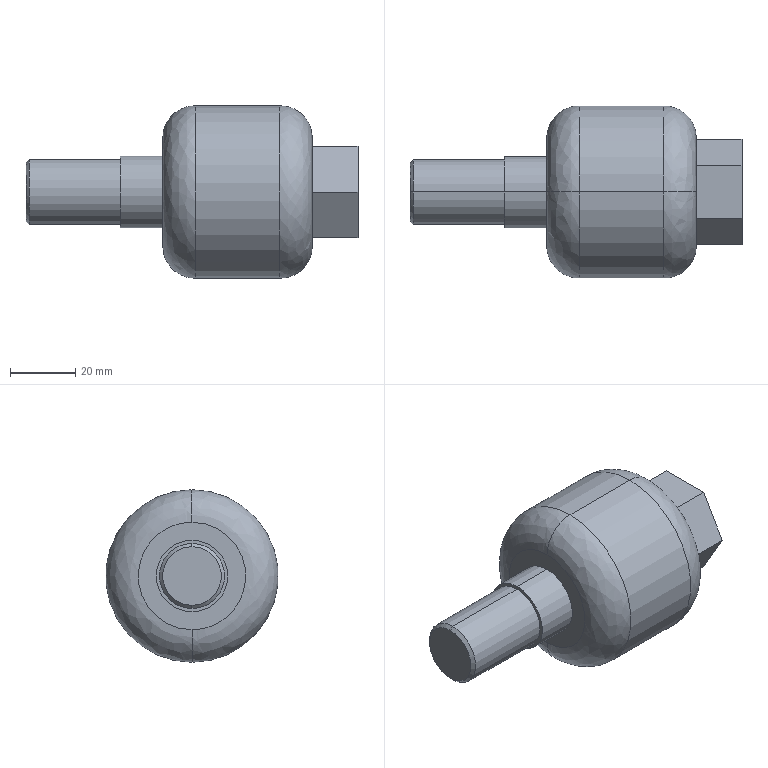Part | STEP file | FJ1020 Floating Joint | 1 solid | 26 faces | box 102 x 53 x 53 mm | volume 114072 mm3 | plane 12 | cylinder 8 | spline 4 | cone 2 | commonest cylinder face diameters 20 x4 22 x2 53 x2
STEP:
#1=CARTESIAN_POINT('',(10.,0.,26.5));
#2=VERTEX_POINT('',#1);
#3=CARTESIAN_POINT('',(10.,0.,-26.5));
#4=VERTEX_POINT('',#3);
#5=CARTESIAN_POINT('',(10.,0.,0.));
#6=DIRECTION('',(1.,0.,0.));
#7=DIRECTION('',(0.,0.,1.));
#8=AXIS2_PLACEMENT_3D('',#5,#6,#7);
#9=CIRCLE('',#8,26.5);
#10=EDGE_CURVE('',#2,#4,#9,.T.);
#11=ORIENTED_EDGE('',*,*,#10,.F.);
#12=CARTESIAN_POINT('',(0.,0.,16.5));
#13=VERTEX_POINT('',#12);
#14=CARTESIAN_POINT('',(10.,0.,16.5));
#15=DIRECTION('',(0.,-1.,0.));
#16=DIRECTION('',(0.,0.,1.));
#17=AXIS2_PLACEMENT_3D('',#14,#15,#16);
#18=CIRCLE('',#17,10.);
#19=EDGE_CURVE('',#2,#13,#18,.T.);
#20=ORIENTED_EDGE('',*,*,#19,.T.);
#21=CARTESIAN_POINT('',(0.,0.,-16.5));
#22=VERTEX_POINT('',#21);
#23=CARTESIAN_POINT('',(0.,0.,16.5));
#24=CARTESIAN_POINT('',(0.,-33.,16.5));
#25=CARTESIAN_POINT('',(0.,-33.,-16.5));
#26=CARTESIAN_POINT('',(0.,0.,-16.5));
#27=(BOUNDED_CURVE()B_SPLINE_CURVE(3,(#23,#24,#25,#26),.UNSPECIFIED.,.F.,.F.)B_SPLINE_CURVE_WITH_KNOTS((4,4),(0.,1.),.UNSPECIFIED.)CURVE()GEOMETRIC_REPRESENTATION_ITEM()RATIONAL_B_SPLINE_CURVE((1.,0.3333,0.3333,1.))REPRESENTATION_ITEM(''));
#28=EDGE_CURVE('',#13,#22,#27,.T.);
#29=ORIENTED_EDGE('',*,*,#28,.T.);
#30=CARTESIAN_POINT('',(10.,0.,-16.5));
#31=DIRECTION('',(0.,1.,0.));
#32=DIRECTION('',(0.,0.,-1.));
#33=AXIS2_PLACEMENT_3D('',#30,#31,#32);
#34=CIRCLE('',#33,10.);
#35=EDGE_CURVE('',#4,#22,#34,.T.);
#36=ORIENTED_EDGE('',*,*,#35,.F.);
#37=EDGE_LOOP('',(#11,#20,#29,#36));
#38=FACE_OUTER_BOUND('',#37,.T.);
#39=CARTESIAN_POINT('',(10.,0.,26.5));
#40=CARTESIAN_POINT('',(10.,-53.,26.5));
#41=CARTESIAN_POINT('',(10.,-53.,-26.5));
#42=CARTESIAN_POINT('',(10.,0.,-26.5));
#43=CARTESIAN_POINT('',(4.142,0.,26.5));
#44=CARTESIAN_POINT('',(4.142,-53.,26.5));
#45=CARTESIAN_POINT('',(4.142,-53.,-26.5));
#46=CARTESIAN_POINT('',(4.142,0.,-26.5));
#47=CARTESIAN_POINT('',(0.,0.,22.358));
#48=CARTESIAN_POINT('',(0.,-44.716,22.358));
#49=CARTESIAN_POINT('',(0.,-44.716,-22.358));
#50=CARTESIAN_POINT('',(0.,0.,-22.358));
#51=CARTESIAN_POINT('',(0.,0.,16.5));
#52=CARTESIAN_POINT('',(0.,-33.,16.5));
#53=CARTESIAN_POINT('',(0.,-33.,-16.5));
#54=CARTESIAN_POINT('',(0.,0.,-16.5));
#55=(BOUNDED_SURFACE()B_SPLINE_SURFACE(3,3,((#39,#40,#41,#42),(#43,#44,#45,#46),(#47,#48,#49,#50),(#51,#52,#53,#54)),.UNSPECIFIED.,.F.,.F.,.F.)B_SPLINE_SURFACE_WITH_KNOTS((4,4),(4,4),(0.,1.),(0.,1.),.UNSPECIFIED.)GEOMETRIC_REPRESENTATION_ITEM()RATIONAL_B_SPLINE_SURFACE(((1.,0.3333,0.3333,1.),(0.8047,0.2682,0.2682,0.8047),(0.8047,0.2682,0.2682,0.8047),(1.,0.3333,0.3333,1.)))REPRESENTATION_ITEM('')SURFACE());
#56=ADVANCED_FACE('',(#38),#55,.T.);
#57=CARTESIAN_POINT('',(46.,0.,-16.5));
#58=VERTEX_POINT('',#57);
#59=CARTESIAN_POINT('',(46.,0.,16.5));
#60=VERTEX_POINT('',#59);
#61=CARTESIAN_POINT('',(46.,0.,-16.5));
#62=CARTESIAN_POINT('',(46.,-33.,-16.5));
#63=CARTESIAN_POINT('',(46.,-33.,16.5));
#64=CARTESIAN_POINT('',(46.,0.,16.5));
#65=(BOUNDED_CURVE()B_SPLINE_CURVE(3,(#61,#62,#63,#64),.UNSPECIFIED.,.F.,.F.)B_SPLINE_CURVE_WITH_KNOTS((4,4),(0.,1.),.UNSPECIFIED.)CURVE()GEOMETRIC_REPRESENTATION_ITEM()RATIONAL_B_SPLINE_CURVE((1.,0.3333,0.3333,1.))REPRESENTATION_ITEM(''));
#66=EDGE_CURVE('',#58,#60,#65,.T.);
#67=ORIENTED_EDGE('',*,*,#66,.T.);
#68=CARTESIAN_POINT('',(36.,0.,26.5));
#69=VERTEX_POINT('',#68);
#70=CARTESIAN_POINT('',(36.,0.,16.5));
#71=DIRECTION('',(0.,-1.,0.));
#72=DIRECTION('',(0.,0.,1.));
#73=AXIS2_PLACEMENT_3D('',#70,#71,#72);
#74=CIRCLE('',#73,10.);
#75=EDGE_CURVE('',#60,#69,#74,.T.);
#76=ORIENTED_EDGE('',*,*,#75,.T.);
#77=CARTESIAN_POINT('',(36.,0.,-26.5));
#78=VERTEX_POINT('',#77);
#79=CARTESIAN_POINT('',(36.,0.,0.));
#80=DIRECTION('',(-1.,0.,0.));
#81=DIRECTION('',(0.,0.,1.));
#82=AXIS2_PLACEMENT_3D('',#79,#80,#81);
#83=CIRCLE('',#82,26.5);
#84=EDGE_CURVE('',#78,#69,#83,.T.);
#85=ORIENTED_EDGE('',*,*,#84,.F.);
#86=CARTESIAN_POINT('',(36.,0.,-16.5));
#87=DIRECTION('',(0.,1.,0.));
#88=DIRECTION('',(0.,0.,-1.));
#89=AXIS2_PLACEMENT_3D('',#86,#87,#88);
#90=CIRCLE('',#89,10.);
#91=EDGE_CURVE('',#58,#78,#90,.T.);
#92=ORIENTED_EDGE('',*,*,#91,.F.);
#93=EDGE_LOOP('',(#67,#76,#85,#92));
#94=FACE_OUTER_BOUND('',#93,.T.);
#95=CARTESIAN_POINT('',(46.,0.,16.5));
#96=CARTESIAN_POINT('',(46.,-33.,16.5));
#97=CARTESIAN_POINT('',(46.,-33.,-16.5));
#98=CARTESIAN_POINT('',(46.,0.,-16.5));
#99=CARTESIAN_POINT('',(46.,0.,22.358));
#100=CARTESIAN_POINT('',(46.,-44.716,22.358));
#101=CARTESIAN_POINT('',(46.,-44.716,-22.358));
#102=CARTESIAN_POINT('',(46.,0.,-22.358));
#103=CARTESIAN_POINT('',(41.858,0.,26.5));
#104=CARTESIAN_POINT('',(41.858,-53.,26.5));
#105=CARTESIAN_POINT('',(41.858,-53.,-26.5));
#106=CARTESIAN_POINT('',(41.858,0.,-26.5));
#107=CARTESIAN_POINT('',(36.,0.,26.5));
#108=CARTESIAN_POINT('',(36.,-53.,26.5));
#109=CARTESIAN_POINT('',(36.,-53.,-26.5));
#110=CARTESIAN_POINT('',(36.,0.,-26.5));
#111=(BOUNDED_SURFACE()B_SPLINE_SURFACE(3,3,((#95,#96,#97,#98),(#99,#100,#101,#102),(#103,#104,#105,#106),(#107,#108,#109,#110)),.UNSPECIFIED.,.F.,.F.,.T.)B_SPLINE_SURFACE_WITH_KNOTS((4,4),(4,4),(0.,1.),(0.,1.),.UNSPECIFIED.)GEOMETRIC_REPRESENTATION_ITEM()RATIONAL_B_SPLINE_SURFACE(((1.,0.3333,0.3333,1.),(0.8047,0.2682,0.2682,0.8047),(0.8047,0.2682,0.2682,0.8047),(1.,0.3333,0.3333,1.)))REPRESENTATION_ITEM('')SURFACE());
#112=ADVANCED_FACE('',(#94),#111,.T.);
#113=CARTESIAN_POINT('',(36.,0.,0.));
#114=DIRECTION('',(-1.,0.,0.));
#115=DIRECTION('',(0.,0.,1.));
#116=AXIS2_PLACEMENT_3D('',#113,#114,#115);
#117=CIRCLE('',#116,26.5);
#118=EDGE_CURVE('',#69,#78,#117,.T.);
#119=ORIENTED_EDGE('',*,*,#118,.T.);
#120=CARTESIAN_POINT('',(46.,0.,-26.5));
#121=DIRECTION('',(-1.,0.,0.));
#122=VECTOR('',#121,1000.);
#123=LINE('',#120,#122);
#124=EDGE_CURVE('',#78,#4,#123,.T.);
#125=ORIENTED_EDGE('',*,*,#124,.T.);
#126=CARTESIAN_POINT('',(10.,0.,0.));
#127=DIRECTION('',(1.,0.,0.));
#128=DIRECTION('',(0.,0.,1.));
#129=AXIS2_PLACEMENT_3D('',#126,#127,#128);
#130=CIRCLE('',#129,26.5);
#131=EDGE_CURVE('',#4,#2,#130,.T.);
#132=ORIENTED_EDGE('',*,*,#131,.T.);
#133=CARTESIAN_POINT('',(46.,0.,26.5));
#134=DIRECTION('',(-1.,0.,0.));
#135=VECTOR('',#134,1000.);
#136=LINE('',#133,#135);
#137=EDGE_CURVE('',#69,#2,#136,.T.);
#138=ORIENTED_EDGE('',*,*,#137,.F.);
#139=EDGE_LOOP('',(#119,#125,#132,#138));
#140=FACE_OUTER_BOUND('',#139,.T.);
#141=CARTESIAN_POINT('',(46.,0.,0.));
#142=DIRECTION('',(-1.,0.,0.));
#143=DIRECTION('',(0.,0.,1.));
#144=AXIS2_PLACEMENT_3D('',#141,#142,#143);
#145=CYLINDRICAL_SURFACE('',#144,26.5);
#146=ADVANCED_FACE('',(#140),#145,.T.);
#147=CARTESIAN_POINT('',(-13.,0.,-11.));
#148=VERTEX_POINT('',#147);
#149=CARTESIAN_POINT('',(-13.,0.,11.));
#150=VERTEX_POINT('',#149);
#151=CARTESIAN_POINT('',(-13.,0.,0.));
#152=DIRECTION('',(1.,0.,0.));
#153=DIRECTION('',(0.,0.,-1.));
#154=AXIS2_PLACEMENT_3D('',#151,#152,#153);
#155=CIRCLE('',#154,11.);
#156=EDGE_CURVE('',#148,#150,#155,.T.);
#157=ORIENTED_EDGE('',*,*,#156,.T.);
#158=CARTESIAN_POINT('',(0.,0.,11.));
#159=VERTEX_POINT('',#158);
#160=CARTESIAN_POINT('',(-13.,0.,11.));
#161=DIRECTION('',(1.,0.,0.));
#162=VECTOR('',#161,1000.);
#163=LINE('',#160,#162);
#164=EDGE_CURVE('',#150,#159,#163,.T.);
#165=ORIENTED_EDGE('',*,*,#164,.T.);
#166=CARTESIAN_POINT('',(0.,0.,-11.));
#167=VERTEX_POINT('',#166);
#168=CARTESIAN_POINT('',(0.,0.,0.));
#169=DIRECTION('',(-1.,0.,0.));
#170=DIRECTION('',(0.,0.,-1.));
#171=AXIS2_PLACEMENT_3D('',#168,#169,#170);
#172=CIRCLE('',#171,11.);
#173=EDGE_CURVE('',#159,#167,#172,.T.);
#174=ORIENTED_EDGE('',*,*,#173,.T.);
#175=CARTESIAN_POINT('',(-13.,0.,-11.));
#176=DIRECTION('',(1.,0.,0.));
#177=VECTOR('',#176,1000.);
#178=LINE('',#175,#177);
#179=EDGE_CURVE('',#148,#167,#178,.T.);
#180=ORIENTED_EDGE('',*,*,#179,.F.);
#181=EDGE_LOOP('',(#157,#165,#174,#180));
#182=FACE_OUTER_BOUND('',#181,.T.);
#183=CARTESIAN_POINT('',(-13.,0.,0.));
#184=DIRECTION('',(1.,0.,0.));
#185=DIRECTION('',(0.,0.,-1.));
#186=AXIS2_PLACEMENT_3D('',#183,#184,#185);
#187=CYLINDRICAL_SURFACE('',#186,11.);
#188=ADVANCED_FACE('',(#182),#187,.T.);
#189=CARTESIAN_POINT('',(-41.,0.,-10.));
#190=VERTEX_POINT('',#189);
#191=CARTESIAN_POINT('',(-41.,0.,10.));
#192=VERTEX_POINT('',#191);
#193=CARTESIAN_POINT('',(-41.,0.,0.));
#194=DIRECTION('',(1.,0.,0.));
#195=DIRECTION('',(0.,0.,-1.));
#196=AXIS2_PLACEMENT_3D('',#193,#194,#195);
#197=CIRCLE('',#196,10.);
#198=EDGE_CURVE('',#190,#192,#197,.T.);
#199=ORIENTED_EDGE('',*,*,#198,.T.);
#200=CARTESIAN_POINT('',(-13.,0.,10.));
#201=VERTEX_POINT('',#200);
#202=CARTESIAN_POINT('',(-42.,0.,10.));
#203=DIRECTION('',(1.,0.,0.));
#204=VECTOR('',#203,1000.);
#205=LINE('',#202,#204);
#206=EDGE_CURVE('',#192,#201,#205,.T.);
#207=ORIENTED_EDGE('',*,*,#206,.T.);
#208=CARTESIAN_POINT('',(-13.,0.,-10.));
#209=VERTEX_POINT('',#208);
#210=CARTESIAN_POINT('',(-13.,0.,0.));
#211=DIRECTION('',(1.,0.,0.));
#212=DIRECTION('',(0.,0.,-1.));
#213=AXIS2_PLACEMENT_3D('',#210,#211,#212);
#214=CIRCLE('',#213,10.);
#215=EDGE_CURVE('',#209,#201,#214,.T.);
#216=ORIENTED_EDGE('',*,*,#215,.F.);
#217=CARTESIAN_POINT('',(-42.,0.,-10.));
#218=DIRECTION('',(1.,0.,0.));
#219=VECTOR('',#218,1000.);
#220=LINE('',#217,#219);
#221=EDGE_CURVE('',#190,#209,#220,.T.);
#222=ORIENTED_EDGE('',*,*,#221,.F.);
#223=EDGE_LOOP('',(#199,#207,#216,#222));
#224=FACE_OUTER_BOUND('',#223,.T.);
#225=CARTESIAN_POINT('',(-42.,0.,0.));
#226=DIRECTION('',(1.,0.,0.));
#227=DIRECTION('',(0.,0.,-1.));
#228=AXIS2_PLACEMENT_3D('',#225,#226,#227);
#229=CYLINDRICAL_SURFACE('',#228,10.);
#230=ADVANCED_FACE('',(#224),#229,.T.);
#231=CARTESIAN_POINT('',(60.,0.,-10.));
#232=VERTEX_POINT('',#231);
#233=CARTESIAN_POINT('',(60.,0.,10.));
#234=VERTEX_POINT('',#233);
#235=CARTESIAN_POINT('',(60.,0.,0.));
#236=DIRECTION('',(-1.,0.,0.));
#237=DIRECTION('',(0.,0.,1.));
#238=AXIS2_PLACEMENT_3D('',#235,#236,#237);
#239=CIRCLE('',#238,10.);
#240=EDGE_CURVE('',#232,#234,#239,.T.);
#241=ORIENTED_EDGE('',*,*,#240,.F.);
#242=CARTESIAN_POINT('',(46.,0.,-10.));
#243=VERTEX_POINT('',#242);
#244=CARTESIAN_POINT('',(60.,0.,-10.));
#245=DIRECTION('',(-1.,0.,0.));
#246=VECTOR('',#245,1000.);
#247=LINE('',#244,#246);
#248=EDGE_CURVE('',#232,#243,#247,.T.);
#249=ORIENTED_EDGE('',*,*,#248,.T.);
#250=CARTESIAN_POINT('',(46.,0.,10.));
#251=VERTEX_POINT('',#250);
#252=CARTESIAN_POINT('',(46.,0.,0.));
#253=DIRECTION('',(1.,0.,0.));
#254=DIRECTION('',(0.,0.,1.));
#255=AXIS2_PLACEMENT_3D('',#252,#253,#254);
#256=CIRCLE('',#255,10.);
#257=EDGE_CURVE('',#251,#243,#256,.T.);
#258=ORIENTED_EDGE('',*,*,#257,.F.);
#259=CARTESIAN_POINT('',(60.,0.,10.));
#260=DIRECTION('',(-1.,0.,0.));
#261=VECTOR('',#260,1000.);
#262=LINE('',#259,#261);
#263=EDGE_CURVE('',#234,#251,#262,.T.);
#264=ORIENTED_EDGE('',*,*,#263,.F.);
#265=EDGE_LOOP('',(#241,#249,#258,#264));
#266=FACE_OUTER_BOUND('',#265,.T.);
#267=CARTESIAN_POINT('',(60.,0.,0.));
#268=DIRECTION('',(-1.,0.,0.));
#269=DIRECTION('',(0.,0.,1.));
#270=AXIS2_PLACEMENT_3D('',#267,#268,#269);
#271=CYLINDRICAL_SURFACE('',#270,10.);
#272=ADVANCED_FACE('',(#266),#271,.F.);
#273=CARTESIAN_POINT('',(-42.,0.,-9.));
#274=VERTEX_POINT('',#273);
#275=CARTESIAN_POINT('',(-42.,0.,9.));
#276=VERTEX_POINT('',#275);
#277=CARTESIAN_POINT('',(-42.,0.,0.));
#278=DIRECTION('',(1.,0.,0.));
#279=DIRECTION('',(0.,0.,-1.));
#280=AXIS2_PLACEMENT_3D('',#277,#278,#279);
#281=CIRCLE('',#280,9.);
#282=EDGE_CURVE('',#274,#276,#281,.T.);
#283=ORIENTED_EDGE('',*,*,#282,.T.);
#284=CARTESIAN_POINT('',(-41.,0.,10.));
#285=DIRECTION('',(0.7071,0.,0.7071));
#286=VECTOR('',#285,1000.);
#287=LINE('',#284,#286);
#288=EDGE_CURVE('',#276,#192,#287,.T.);
#289=ORIENTED_EDGE('',*,*,#288,.T.);
#290=ORIENTED_EDGE('',*,*,#198,.F.);
#291=CARTESIAN_POINT('',(-41.,0.,-10.));
#292=DIRECTION('',(0.7071,0.,-0.7071));
#293=VECTOR('',#292,1000.);
#294=LINE('',#291,#293);
#295=EDGE_CURVE('',#274,#190,#294,.T.);
#296=ORIENTED_EDGE('',*,*,#295,.F.);
#297=EDGE_LOOP('',(#283,#289,#290,#296));
#298=FACE_OUTER_BOUND('',#297,.T.);
#299=CARTESIAN_POINT('',(-41.,0.,0.));
#300=DIRECTION('',(1.,0.,0.));
#301=DIRECTION('',(0.,0.,-1.));
#302=AXIS2_PLACEMENT_3D('',#299,#300,#301);
#303=CONICAL_SURFACE('',#302,10.,0.7854);
#304=ADVANCED_FACE('',(#298),#303,.T.);
#305=ORIENTED_EDGE('',*,*,#124,.F.);
#306=ORIENTED_EDGE('',*,*,#84,.T.);
#307=ORIENTED_EDGE('',*,*,#137,.T.);
#308=ORIENTED_EDGE('',*,*,#10,.T.);
#309=EDGE_LOOP('',(#305,#306,#307,#308));
#310=FACE_OUTER_BOUND('',#309,.T.);
#311=CARTESIAN_POINT('',(46.,0.,0.));
#312=DIRECTION('',(-1.,0.,0.));
#313=DIRECTION('',(0.,0.,1.));
#314=AXIS2_PLACEMENT_3D('',#311,#312,#313);
#315=CYLINDRICAL_SURFACE('',#314,26.5);
#316=ADVANCED_FACE('',(#310),#315,.T.);
#317=ORIENTED_EDGE('',*,*,#19,.F.);
#318=ORIENTED_EDGE('',*,*,#131,.F.);
#319=ORIENTED_EDGE('',*,*,#35,.T.);
#320=CARTESIAN_POINT('',(0.,0.,-16.5));
#321=CARTESIAN_POINT('',(0.,33.,-16.5));
#322=CARTESIAN_POINT('',(0.,33.,16.5));
#323=CARTESIAN_POINT('',(0.,0.,16.5));
#324=(BOUNDED_CURVE()B_SPLINE_CURVE(3,(#320,#321,#322,#323),.UNSPECIFIED.,.F.,.F.)B_SPLINE_CURVE_WITH_KNOTS((4,4),(0.,1.),.UNSPECIFIED.)CURVE()GEOMETRIC_REPRESENTATION_ITEM()RATIONAL_B_SPLINE_CURVE((1.,0.3333,0.3333,1.))REPRESENTATION_ITEM(''));
#325=EDGE_CURVE('',#22,#13,#324,.T.);
#326=ORIENTED_EDGE('',*,*,#325,.T.);
#327=EDGE_LOOP('',(#317,#318,#319,#326));
#328=FACE_OUTER_BOUND('',#327,.T.);
#329=CARTESIAN_POINT('',(10.,0.,-26.5));
#330=CARTESIAN_POINT('',(10.,53.,-26.5));
#331=CARTESIAN_POINT('',(10.,53.,26.5));
#332=CARTESIAN_POINT('',(10.,0.,26.5));
#333=CARTESIAN_POINT('',(4.142,0.,-26.5));
#334=CARTESIAN_POINT('',(4.142,53.,-26.5));
#335=CARTESIAN_POINT('',(4.142,53.,26.5));
#336=CARTESIAN_POINT('',(4.142,0.,26.5));
#337=CARTESIAN_POINT('',(0.,0.,-22.358));
#338=CARTESIAN_POINT('',(0.,44.716,-22.358));
#339=CARTESIAN_POINT('',(0.,44.716,22.358));
#340=CARTESIAN_POINT('',(0.,0.,22.358));
#341=CARTESIAN_POINT('',(0.,0.,-16.5));
#342=CARTESIAN_POINT('',(0.,33.,-16.5));
#343=CARTESIAN_POINT('',(0.,33.,16.5));
#344=CARTESIAN_POINT('',(0.,0.,16.5));
#345=(BOUNDED_SURFACE()B_SPLINE_SURFACE(3,3,((#329,#330,#331,#332),(#333,#334,#335,#336),(#337,#338,#339,#340),(#341,#342,#343,#344)),.UNSPECIFIED.,.F.,.F.,.F.)B_SPLINE_SURFACE_WITH_KNOTS((4,4),(4,4),(0.,1.),(0.,1.),.UNSPECIFIED.)GEOMETRIC_REPRESENTATION_ITEM()RATIONAL_B_SPLINE_SURFACE(((1.,0.3333,0.3333,1.),(0.8047,0.2682,0.2682,0.8047),(0.8047,0.2682,0.2682,0.8047),(1.,0.3333,0.3333,1.)))REPRESENTATION_ITEM('')SURFACE());
#346=ADVANCED_FACE('',(#328),#345,.T.);
#347=ORIENTED_EDGE('',*,*,#75,.F.);
#348=CARTESIAN_POINT('',(46.,0.,16.5));
#349=CARTESIAN_POINT('',(46.,33.,16.5));
#350=CARTESIAN_POINT('',(46.,33.,-16.5));
#351=CARTESIAN_POINT('',(46.,0.,-16.5));
#352=(BOUNDED_CURVE()B_SPLINE_CURVE(3,(#348,#349,#350,#351),.UNSPECIFIED.,.F.,.F.)B_SPLINE_CURVE_WITH_KNOTS((4,4),(0.,1.),.UNSPECIFIED.)CURVE()GEOMETRIC_REPRESENTATION_ITEM()RATIONAL_B_SPLINE_CURVE((1.,0.3333,0.3333,1.))REPRESENTATION_ITEM(''));
#353=EDGE_CURVE('',#60,#58,#352,.T.);
#354=ORIENTED_EDGE('',*,*,#353,.T.);
#355=ORIENTED_EDGE('',*,*,#91,.T.);
#356=ORIENTED_EDGE('',*,*,#118,.F.);
#357=EDGE_LOOP('',(#347,#354,#355,#356));
#358=FACE_OUTER_BOUND('',#357,.T.);
#359=CARTESIAN_POINT('',(46.,0.,-16.5));
#360=CARTESIAN_POINT('',(46.,33.,-16.5));
#361=CARTESIAN_POINT('',(46.,33.,16.5));
#362=CARTESIAN_POINT('',(46.,0.,16.5));
#363=CARTESIAN_POINT('',(46.,0.,-22.358));
#364=CARTESIAN_POINT('',(46.,44.716,-22.358));
#365=CARTESIAN_POINT('',(46.,44.716,22.358));
#366=CARTESIAN_POINT('',(46.,0.,22.358));
#367=CARTESIAN_POINT('',(41.858,0.,-26.5));
#368=CARTESIAN_POINT('',(41.858,53.,-26.5));
#369=CARTESIAN_POINT('',(41.858,53.,26.5));
#370=CARTESIAN_POINT('',(41.858,0.,26.5));
#371=CARTESIAN_POINT('',(36.,0.,-26.5));
#372=CARTESIAN_POINT('',(36.,53.,-26.5));
#373=CARTESIAN_POINT('',(36.,53.,26.5));
#374=CARTESIAN_POINT('',(36.,0.,26.5));
#375=(BOUNDED_SURFACE()B_SPLINE_SURFACE(3,3,((#359,#360,#361,#362),(#363,#364,#365,#366),(#367,#368,#369,#370),(#371,#372,#373,#374)),.UNSPECIFIED.,.F.,.F.,.F.)B_SPLINE_SURFACE_WITH_KNOTS((4,4),(4,4),(0.,1.),(0.,1.),.UNSPECIFIED.)GEOMETRIC_REPRESENTATION_ITEM()RATIONAL_B_SPLINE_SURFACE(((1.,0.3333,0.3333,1.),(0.8047,0.2682,0.2682,0.8047),(0.8047,0.2682,0.2682,0.8047),(1.,0.3333,0.3333,1.)))REPRESENTATION_ITEM('')SURFACE());
#376=ADVANCED_FACE('',(#358),#375,.T.);
#377=CARTESIAN_POINT('',(0.,0.,0.));
#378=DIRECTION('',(-1.,0.,0.));
#379=DIRECTION('',(0.,0.,-1.));
#380=AXIS2_PLACEMENT_3D('',#377,#378,#379);
#381=CIRCLE('',#380,11.);
#382=EDGE_CURVE('',#167,#159,#381,.T.);
#383=ORIENTED_EDGE('',*,*,#382,.F.);
#384=ORIENTED_EDGE('',*,*,#173,.F.);
#385=EDGE_LOOP('',(#383,#384));
#386=FACE_BOUND('',#385,.T.);
#387=ORIENTED_EDGE('',*,*,#325,.F.);
#388=ORIENTED_EDGE('',*,*,#28,.F.);
#389=EDGE_LOOP('',(#387,#388));
#390=FACE_OUTER_BOUND('',#389,.T.);
#391=CARTESIAN_POINT('',(0.,0.,0.));
#392=DIRECTION('',(1.,0.,0.));
#393=DIRECTION('',(0.,0.,-1.));
#394=AXIS2_PLACEMENT_3D('',#391,#392,#393);
#395=PLANE('',#394);
#396=ADVANCED_FACE('',(#386,#390),#395,.F.);
#397=CARTESIAN_POINT('',(46.,-16.166,0.));
#398=VERTEX_POINT('',#397);
#399=CARTESIAN_POINT('',(46.,-8.083,14.));
#400=VERTEX_POINT('',#399);
#401=CARTESIAN_POINT('',(46.,-16.166,0.));
#402=DIRECTION('',(0.,0.5,0.866));
#403=VECTOR('',#402,1000.);
#404=LINE('',#401,#403);
#405=EDGE_CURVE('',#398,#400,#404,.T.);
#406=ORIENTED_EDGE('',*,*,#405,.T.);
#407=CARTESIAN_POINT('',(46.,8.083,14.));
#408=VERTEX_POINT('',#407);
#409=CARTESIAN_POINT('',(46.,0.,14.));
#410=DIRECTION('',(0.,1.,0.));
#411=VECTOR('',#410,1000.);
#412=LINE('',#409,#411);
#413=EDGE_CURVE('',#400,#408,#412,.T.);
#414=ORIENTED_EDGE('',*,*,#413,.T.);
#415=CARTESIAN_POINT('',(46.,16.166,0.));
#416=VERTEX_POINT('',#415);
#417=CARTESIAN_POINT('',(46.,8.083,14.));
#418=DIRECTION('',(0.,0.5,-0.866));
#419=VECTOR('',#418,1000.);
#420=LINE('',#417,#419);
#421=EDGE_CURVE('',#408,#416,#420,.T.);
#422=ORIENTED_EDGE('',*,*,#421,.T.);
#423=CARTESIAN_POINT('',(46.,8.083,-14.));
#424=VERTEX_POINT('',#423);
#425=CARTESIAN_POINT('',(46.,16.166,0.));
#426=DIRECTION('',(0.,-0.5,-0.866));
#427=VECTOR('',#426,1000.);
#428=LINE('',#425,#427);
#429=EDGE_CURVE('',#416,#424,#428,.T.);
#430=ORIENTED_EDGE('',*,*,#429,.T.);
#431=CARTESIAN_POINT('',(46.,-8.083,-14.));
#432=VERTEX_POINT('',#431);
#433=CARTESIAN_POINT('',(46.,0.,-14.));
#434=DIRECTION('',(0.,-1.,0.));
#435=VECTOR('',#434,1000.);
#436=LINE('',#433,#435);
#437=EDGE_CURVE('',#424,#432,#436,.T.);
#438=ORIENTED_EDGE('',*,*,#437,.T.);
#439=CARTESIAN_POINT('',(46.,-8.083,-14.));
#440=DIRECTION('',(0.,-0.5,0.866));
#441=VECTOR('',#440,1000.);
#442=LINE('',#439,#441);
#443=EDGE_CURVE('',#432,#398,#442,.T.);
#444=ORIENTED_EDGE('',*,*,#443,.T.);
#445=EDGE_LOOP('',(#406,#414,#422,#430,#438,#444));
#446=FACE_BOUND('',#445,.T.);
#447=ORIENTED_EDGE('',*,*,#353,.F.);
#448=ORIENTED_EDGE('',*,*,#66,.F.);
#449=EDGE_LOOP('',(#447,#448));
#450=FACE_OUTER_BOUND('',#449,.T.);
#451=CARTESIAN_POINT('',(46.,0.,0.));
#452=DIRECTION('',(1.,0.,0.));
#453=DIRECTION('',(0.,0.,-1.));
#454=AXIS2_PLACEMENT_3D('',#451,#452,#453);
#455=PLANE('',#454);
#456=ADVANCED_FACE('',(#446,#450),#455,.T.);
#457=ORIENTED_EDGE('',*,*,#164,.F.);
#458=CARTESIAN_POINT('',(-13.,0.,0.));
#459=DIRECTION('',(1.,0.,0.));
#460=DIRECTION('',(0.,0.,-1.));
#461=AXIS2_PLACEMENT_3D('',#458,#459,#460);
#462=CIRCLE('',#461,11.);
#463=EDGE_CURVE('',#150,#148,#462,.T.);
#464=ORIENTED_EDGE('',*,*,#463,.T.);
#465=ORIENTED_EDGE('',*,*,#179,.T.);
#466=ORIENTED_EDGE('',*,*,#382,.T.);
#467=EDGE_LOOP('',(#457,#464,#465,#466));
#468=FACE_OUTER_BOUND('',#467,.T.);
#469=CARTESIAN_POINT('',(-13.,0.,0.));
#470=DIRECTION('',(1.,0.,0.));
#471=DIRECTION('',(0.,0.,-1.));
#472=AXIS2_PLACEMENT_3D('',#469,#470,#471);
#473=CYLINDRICAL_SURFACE('',#472,11.);
#474=ADVANCED_FACE('',(#468),#473,.T.);
#475=CARTESIAN_POINT('',(60.,-8.083,14.));
#476=VERTEX_POINT('',#475);
#477=CARTESIAN_POINT('',(60.,-8.083,14.));
#478=DIRECTION('',(-1.,0.,0.));
#479=VECTOR('',#478,1000.);
#480=LINE('',#477,#479);
#481=EDGE_CURVE('',#476,#400,#480,.T.);
#482=ORIENTED_EDGE('',*,*,#481,.F.);
#483=CARTESIAN_POINT('',(60.,8.083,14.));
#484=VERTEX_POINT('',#483);
#485=CARTESIAN_POINT('',(60.,8.083,14.));
#486=DIRECTION('',(0.,-1.,0.));
#487=VECTOR('',#486,1000.);
#488=LINE('',#485,#487);
#489=EDGE_CURVE('',#484,#476,#488,.T.);
#490=ORIENTED_EDGE('',*,*,#489,.F.);
#491=CARTESIAN_POINT('',(60.,8.083,14.));
#492=DIRECTION('',(1.,0.,0.));
#493=VECTOR('',#492,1000.);
#494=LINE('',#491,#493);
#495=EDGE_CURVE('',#408,#484,#494,.T.);
#496=ORIENTED_EDGE('',*,*,#495,.F.);
#497=ORIENTED_EDGE('',*,*,#413,.F.);
#498=EDGE_LOOP('',(#482,#490,#496,#497));
#499=FACE_OUTER_BOUND('',#498,.T.);
#500=CARTESIAN_POINT('',(60.,8.083,14.));
#501=DIRECTION('',(0.,0.,-1.));
#502=DIRECTION('',(-1.,0.,0.));
#503=AXIS2_PLACEMENT_3D('',#500,#501,#502);
#504=PLANE('',#503);
#505=ADVANCED_FACE('',(#499),#504,.F.);
#506=CARTESIAN_POINT('',(60.,-16.166,0.));
#507=VERTEX_POINT('',#506);
#508=CARTESIAN_POINT('',(60.,-16.166,0.));
#509=DIRECTION('',(-1.,0.,0.));
#510=VECTOR('',#509,1000.);
#511=LINE('',#508,#510);
#512=EDGE_CURVE('',#507,#398,#511,.T.);
#513=ORIENTED_EDGE('',*,*,#512,.F.);
#514=CARTESIAN_POINT('',(60.,-8.083,14.));
#515=DIRECTION('',(0.,-0.5,-0.866));
#516=VECTOR('',#515,1000.);
#517=LINE('',#514,#516);
#518=EDGE_CURVE('',#476,#507,#517,.T.);
#519=ORIENTED_EDGE('',*,*,#518,.F.);
#520=ORIENTED_EDGE('',*,*,#481,.T.);
#521=ORIENTED_EDGE('',*,*,#405,.F.);
#522=EDGE_LOOP('',(#513,#519,#520,#521));
#523=FACE_OUTER_BOUND('',#522,.T.);
#524=CARTESIAN_POINT('',(60.,-8.083,14.));
#525=DIRECTION('',(0.,0.866,-0.5));
#526=DIRECTION('',(0.,0.5,0.866));
#527=AXIS2_PLACEMENT_3D('',#524,#525,#526);
#528=PLANE('',#527);
#529=ADVANCED_FACE('',(#523),#528,.F.);
#530=CARTESIAN_POINT('',(60.,-8.083,-14.));
#531=VERTEX_POINT('',#530);
#532=CARTESIAN_POINT('',(60.,-8.083,-14.));
#533=DIRECTION('',(-1.,0.,0.));
#534=VECTOR('',#533,1000.);
#535=LINE('',#532,#534);
#536=EDGE_CURVE('',#531,#432,#535,.T.);
#537=ORIENTED_EDGE('',*,*,#536,.F.);
#538=CARTESIAN_POINT('',(60.,-16.166,0.));
#539=DIRECTION('',(0.,0.5,-0.866));
#540=VECTOR('',#539,1000.);
#541=LINE('',#538,#540);
#542=EDGE_CURVE('',#507,#531,#541,.T.);
#543=ORIENTED_EDGE('',*,*,#542,.F.);
#544=ORIENTED_EDGE('',*,*,#512,.T.);
#545=ORIENTED_EDGE('',*,*,#443,.F.);
#546=EDGE_LOOP('',(#537,#543,#544,#545));
#547=FACE_OUTER_BOUND('',#546,.T.);
#548=CARTESIAN_POINT('',(60.,-16.166,0.));
#549=DIRECTION('',(0.,0.866,0.5));
#550=DIRECTION('',(0.,-0.5,0.866));
#551=AXIS2_PLACEMENT_3D('',#548,#549,#550);
#552=PLANE('',#551);
#553=ADVANCED_FACE('',(#547),#552,.F.);
#554=CARTESIAN_POINT('',(60.,8.083,-14.));
#555=VERTEX_POINT('',#554);
#556=CARTESIAN_POINT('',(60.,8.083,-14.));
#557=DIRECTION('',(-1.,0.,0.));
#558=VECTOR('',#557,1000.);
#559=LINE('',#556,#558);
#560=EDGE_CURVE('',#555,#424,#559,.T.);
#561=ORIENTED_EDGE('',*,*,#560,.F.);
#562=CARTESIAN_POINT('',(60.,-8.083,-14.));
#563=DIRECTION('',(0.,1.,0.));
#564=VECTOR('',#563,1000.);
#565=LINE('',#562,#564);
#566=EDGE_CURVE('',#531,#555,#565,.T.);
#567=ORIENTED_EDGE('',*,*,#566,.F.);
#568=ORIENTED_EDGE('',*,*,#536,.T.);
#569=ORIENTED_EDGE('',*,*,#437,.F.);
#570=EDGE_LOOP('',(#561,#567,#568,#569));
#571=FACE_OUTER_BOUND('',#570,.T.);
#572=CARTESIAN_POINT('',(60.,-8.083,-14.));
#573=DIRECTION('',(0.,0.,1.));
#574=DIRECTION('',(0.,-1.,0.));
#575=AXIS2_PLACEMENT_3D('',#572,#573,#574);
#576=PLANE('',#575);
#577=ADVANCED_FACE('',(#571),#576,.F.);
#578=CARTESIAN_POINT('',(60.,16.166,0.));
#579=VERTEX_POINT('',#578);
#580=CARTESIAN_POINT('',(60.,16.166,0.));
#581=DIRECTION('',(-1.,0.,0.));
#582=VECTOR('',#581,1000.);
#583=LINE('',#580,#582);
#584=EDGE_CURVE('',#579,#416,#583,.T.);
#585=ORIENTED_EDGE('',*,*,#584,.F.);
#586=CARTESIAN_POINT('',(60.,8.083,-14.));
#587=DIRECTION('',(0.,0.5,0.866));
#588=VECTOR('',#587,1000.);
#589=LINE('',#586,#588);
#590=EDGE_CURVE('',#555,#579,#589,.T.);
#591=ORIENTED_EDGE('',*,*,#590,.F.);
#592=ORIENTED_EDGE('',*,*,#560,.T.);
#593=ORIENTED_EDGE('',*,*,#429,.F.);
#594=EDGE_LOOP('',(#585,#591,#592,#593));
#595=FACE_OUTER_BOUND('',#594,.T.);
#596=CARTESIAN_POINT('',(60.,8.083,-14.));
#597=DIRECTION('',(0.,-0.866,0.5));
#598=DIRECTION('',(0.,-0.5,-0.866));
#599=AXIS2_PLACEMENT_3D('',#596,#597,#598);
#600=PLANE('',#599);
#601=ADVANCED_FACE('',(#595),#600,.F.);
#602=ORIENTED_EDGE('',*,*,#495,.T.);
#603=CARTESIAN_POINT('',(60.,16.166,0.));
#604=DIRECTION('',(0.,-0.5,0.866));
#605=VECTOR('',#604,1000.);
#606=LINE('',#603,#605);
#607=EDGE_CURVE('',#579,#484,#606,.T.);
#608=ORIENTED_EDGE('',*,*,#607,.F.);
#609=ORIENTED_EDGE('',*,*,#584,.T.);
#610=ORIENTED_EDGE('',*,*,#421,.F.);
#611=EDGE_LOOP('',(#602,#608,#609,#610));
#612=FACE_OUTER_BOUND('',#611,.T.);
#613=CARTESIAN_POINT('',(60.,16.166,0.));
#614=DIRECTION('',(0.,-0.866,-0.5));
#615=DIRECTION('',(0.,0.5,-0.866));
#616=AXIS2_PLACEMENT_3D('',#613,#614,#615);
#617=PLANE('',#616);
#618=ADVANCED_FACE('',(#612),#617,.F.);
#619=ORIENTED_EDGE('',*,*,#215,.T.);
#620=CARTESIAN_POINT('',(-13.,0.,0.));
#621=DIRECTION('',(1.,0.,0.));
#622=DIRECTION('',(0.,0.,-1.));
#623=AXIS2_PLACEMENT_3D('',#620,#621,#622);
#624=CIRCLE('',#623,10.);
#625=EDGE_CURVE('',#201,#209,#624,.T.);
#626=ORIENTED_EDGE('',*,*,#625,.T.);
#627=EDGE_LOOP('',(#619,#626));
#628=FACE_BOUND('',#627,.T.);
#629=ORIENTED_EDGE('',*,*,#156,.F.);
#630=ORIENTED_EDGE('',*,*,#463,.F.);
#631=EDGE_LOOP('',(#629,#630));
#632=FACE_OUTER_BOUND('',#631,.T.);
#633=CARTESIAN_POINT('',(-13.,0.,0.));
#634=DIRECTION('',(-1.,0.,0.));
#635=DIRECTION('',(0.,0.,1.));
#636=AXIS2_PLACEMENT_3D('',#633,#634,#635);
#637=PLANE('',#636);
#638=ADVANCED_FACE('',(#628,#632),#637,.T.);
#639=CARTESIAN_POINT('',(60.,0.,0.));
#640=DIRECTION('',(-1.,0.,0.));
#641=DIRECTION('',(0.,0.,1.));
#642=AXIS2_PLACEMENT_3D('',#639,#640,#641);
#643=CIRCLE('',#642,10.);
#644=EDGE_CURVE('',#234,#232,#643,.T.);
#645=ORIENTED_EDGE('',*,*,#644,.T.);
#646=ORIENTED_EDGE('',*,*,#240,.T.);
#647=EDGE_LOOP('',(#645,#646));
#648=FACE_BOUND('',#647,.T.);
#649=ORIENTED_EDGE('',*,*,#542,.T.);
#650=ORIENTED_EDGE('',*,*,#566,.T.);
#651=ORIENTED_EDGE('',*,*,#590,.T.);
#652=ORIENTED_EDGE('',*,*,#607,.T.);
#653=ORIENTED_EDGE('',*,*,#489,.T.);
#654=ORIENTED_EDGE('',*,*,#518,.T.);
#655=EDGE_LOOP('',(#649,#650,#651,#652,#653,#654));
#656=FACE_OUTER_BOUND('',#655,.T.);
#657=CARTESIAN_POINT('',(60.,0.,0.));
#658=DIRECTION('',(1.,0.,0.));
#659=DIRECTION('',(0.,0.,-1.));
#660=AXIS2_PLACEMENT_3D('',#657,#658,#659);
#661=PLANE('',#660);
#662=ADVANCED_FACE('',(#648,#656),#661,.T.);
#663=ORIENTED_EDGE('',*,*,#206,.F.);
#664=CARTESIAN_POINT('',(-41.,0.,0.));
#665=DIRECTION('',(1.,0.,0.));
#666=DIRECTION('',(0.,0.,-1.));
#667=AXIS2_PLACEMENT_3D('',#664,#665,#666);
#668=CIRCLE('',#667,10.);
#669=EDGE_CURVE('',#192,#190,#668,.T.);
#670=ORIENTED_EDGE('',*,*,#669,.T.);
#671=ORIENTED_EDGE('',*,*,#221,.T.);
#672=ORIENTED_EDGE('',*,*,#625,.F.);
#673=EDGE_LOOP('',(#663,#670,#671,#672));
#674=FACE_OUTER_BOUND('',#673,.T.);
#675=CARTESIAN_POINT('',(-42.,0.,0.));
#676=DIRECTION('',(1.,0.,0.));
#677=DIRECTION('',(0.,0.,-1.));
#678=AXIS2_PLACEMENT_3D('',#675,#676,#677);
#679=CYLINDRICAL_SURFACE('',#678,10.);
#680=ADVANCED_FACE('',(#674),#679,.T.);
#681=ORIENTED_EDGE('',*,*,#248,.F.);
#682=ORIENTED_EDGE('',*,*,#644,.F.);
#683=ORIENTED_EDGE('',*,*,#263,.T.);
#684=CARTESIAN_POINT('',(46.,0.,0.));
#685=DIRECTION('',(1.,0.,0.));
#686=DIRECTION('',(0.,0.,1.));
#687=AXIS2_PLACEMENT_3D('',#684,#685,#686);
#688=CIRCLE('',#687,10.);
#689=EDGE_CURVE('',#243,#251,#688,.T.);
#690=ORIENTED_EDGE('',*,*,#689,.F.);
#691=EDGE_LOOP('',(#681,#682,#683,#690));
#692=FACE_OUTER_BOUND('',#691,.T.);
#693=CARTESIAN_POINT('',(60.,0.,0.));
#694=DIRECTION('',(-1.,0.,0.));
#695=DIRECTION('',(0.,0.,1.));
#696=AXIS2_PLACEMENT_3D('',#693,#694,#695);
#697=CYLINDRICAL_SURFACE('',#696,10.);
#698=ADVANCED_FACE('',(#692),#697,.F.);
#699=ORIENTED_EDGE('',*,*,#288,.F.);
#700=CARTESIAN_POINT('',(-42.,0.,0.));
#701=DIRECTION('',(1.,0.,0.));
#702=DIRECTION('',(0.,0.,-1.));
#703=AXIS2_PLACEMENT_3D('',#700,#701,#702);
#704=CIRCLE('',#703,9.);
#705=EDGE_CURVE('',#276,#274,#704,.T.);
#706=ORIENTED_EDGE('',*,*,#705,.T.);
#707=ORIENTED_EDGE('',*,*,#295,.T.);
#708=ORIENTED_EDGE('',*,*,#669,.F.);
#709=EDGE_LOOP('',(#699,#706,#707,#708));
#710=FACE_OUTER_BOUND('',#709,.T.);
#711=CARTESIAN_POINT('',(-41.,0.,0.));
#712=DIRECTION('',(1.,0.,0.));
#713=DIRECTION('',(0.,0.,-1.));
#714=AXIS2_PLACEMENT_3D('',#711,#712,#713);
#715=CONICAL_SURFACE('',#714,10.,0.7854);
#716=ADVANCED_FACE('',(#710),#715,.T.);
#717=ORIENTED_EDGE('',*,*,#257,.T.);
#718=ORIENTED_EDGE('',*,*,#689,.T.);
#719=EDGE_LOOP('',(#717,#718));
#720=FACE_OUTER_BOUND('',#719,.T.);
#721=CARTESIAN_POINT('',(46.,0.,0.));
#722=DIRECTION('',(1.,0.,0.));
#723=DIRECTION('',(0.,0.,-1.));
#724=AXIS2_PLACEMENT_3D('',#721,#722,#723);
#725=PLANE('',#724);
#726=ADVANCED_FACE('',(#720),#725,.T.);
#727=ORIENTED_EDGE('',*,*,#282,.F.);
#728=ORIENTED_EDGE('',*,*,#705,.F.);
#729=EDGE_LOOP('',(#727,#728));
#730=FACE_OUTER_BOUND('',#729,.T.);
#731=CARTESIAN_POINT('',(-42.,0.,0.));
#732=DIRECTION('',(-1.,0.,0.));
#733=DIRECTION('',(0.,0.,1.));
#734=AXIS2_PLACEMENT_3D('',#731,#732,#733);
#735=PLANE('',#734);
#736=ADVANCED_FACE('',(#730),#735,.T.);
#737=CLOSED_SHELL('',(#56,#112,#146,#188,#230,#272,#304,#316,#346,#376,#396,#456,#474,#505,#529,#553,#577,#601,#618,#638,#662,#680,#698,#716,#726,#736));
#738=MANIFOLD_SOLID_BREP('',#737);
#739=CARTESIAN_POINT('',(0.,0.,0.));
#740=DIRECTION('',(0.,0.,1.));
#741=DIRECTION('',(1.,0.,0.));
#742=AXIS2_PLACEMENT_3D('',#739,#740,#741);
#743=(LENGTH_UNIT()NAMED_UNIT(*)SI_UNIT(.MILLI.,.METRE.));
#744=UNCERTAINTY_MEASURE_WITH_UNIT(LENGTH_MEASURE(0.00001),#743,'','');
#745=(NAMED_UNIT(*)PLANE_ANGLE_UNIT()SI_UNIT($,.RADIAN.));
#746=(NAMED_UNIT(*)SI_UNIT($,.STERADIAN.)SOLID_ANGLE_UNIT());
#747=(GEOMETRIC_REPRESENTATION_CONTEXT(3)GLOBAL_UNCERTAINTY_ASSIGNED_CONTEXT((#744))GLOBAL_UNIT_ASSIGNED_CONTEXT((#743,#745,#746))REPRESENTATION_CONTEXT('',''));
#748=ADVANCED_BREP_SHAPE_REPRESENTATION('',(#738,#742),#747);